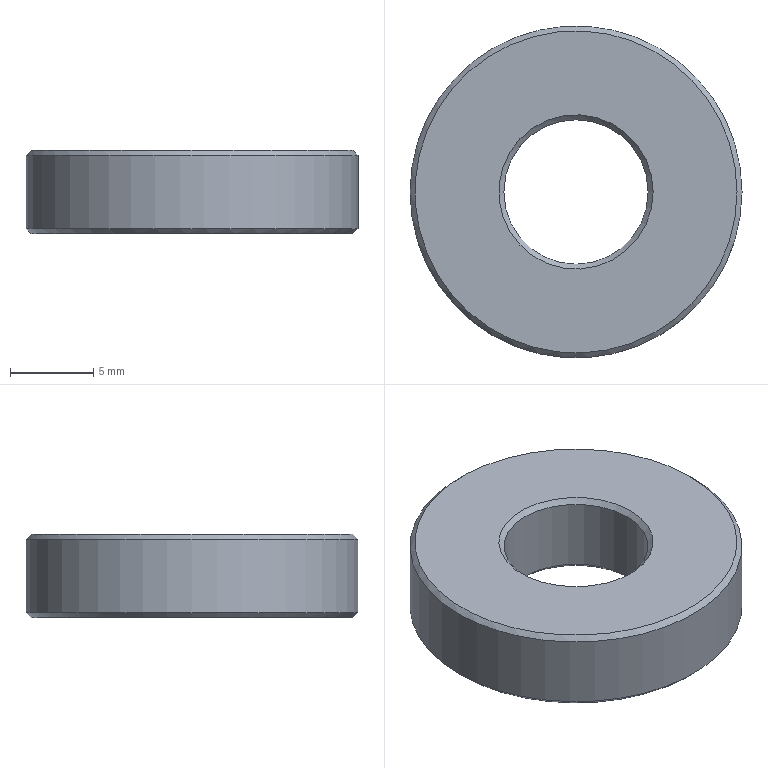Part | STEP file | 1 solid | 8 faces | box 20 x 20 x 5 mm | volume 1265 mm3 | cone 4 | plane 2 | cylinder 2 | commonest cylinder face diameters 8.7 x1 20 x1
STEP:
#1=CARTESIAN_POINT('',(0.,0.,0.));
#2=DIRECTION('',(0.,0.,1.));
#3=DIRECTION('',(1.,0.,0.));
#4=AXIS2_PLACEMENT_3D('',#1,#2,#3);
#5=CARTESIAN_POINT('',(1432.597,532.48,-85.381));
#6=VERTEX_POINT('',#5);
#7=CARTESIAN_POINT('',(1437.247,532.48,-85.381));
#8=DIRECTION('',(0.,0.,1.));
#9=DIRECTION('',(-1.,0.,0.));
#10=AXIS2_PLACEMENT_3D('',#7,#8,#9);
#11=CIRCLE('',#10,4.65);
#12=CARTESIAN_POINT('',(1437.247,532.48,-85.381));
#13=DIRECTION('',(0.,0.,-1.));
#14=DIRECTION('',(1.,0.,0.));
#15=AXIS2_PLACEMENT_3D('',#12,#13,#14);
#16=PLANE('',#15);
#17=CARTESIAN_POINT('',(-4.65,0.));
#18=CARTESIAN_POINT('',(-4.65,8.054));
#19=CARTESIAN_POINT('',(2.325,4.027));
#20=CARTESIAN_POINT('',(9.3,0.));
#21=CARTESIAN_POINT('',(2.325,-4.027));
#22=CARTESIAN_POINT('',(-4.65,-8.054));
#23=CARTESIAN_POINT('',(-4.65,0.));
#24=(BOUNDED_CURVE()B_SPLINE_CURVE(2,(#17,#18,#19,#20,#21,#22,#23),.UNSPECIFIED.,.T.,.F.)B_SPLINE_CURVE_WITH_KNOTS((1,2,2,2,2,1),(-2.094,0.,2.094,4.189,6.283,8.378),.UNSPECIFIED.)CURVE()GEOMETRIC_REPRESENTATION_ITEM()RATIONAL_B_SPLINE_CURVE((1.,0.5,1.,0.5,1.,0.5,1.))REPRESENTATION_ITEM(''));
#25=(GEOMETRIC_REPRESENTATION_CONTEXT(2)PARAMETRIC_REPRESENTATION_CONTEXT()REPRESENTATION_CONTEXT('',''));
#26=DEFINITIONAL_REPRESENTATION('',(#24),#25);
#27=PCURVE('',#16,#26);
#28=CARTESIAN_POINT('',(1437.247,532.48,-85.381));
#29=DIRECTION('',(0.,0.,-1.));
#30=DIRECTION('',(-1.,0.,0.));
#31=AXIS2_PLACEMENT_3D('',#28,#29,#30);
#32=CONICAL_SURFACE('',#31,4.65,0.7854);
#33=CARTESIAN_POINT('',(6.283,0.));
#34=DIRECTION('',(-1.,0.));
#35=VECTOR('',#34,1.);
#36=LINE('',#33,#35);
#37=(GEOMETRIC_REPRESENTATION_CONTEXT(2)PARAMETRIC_REPRESENTATION_CONTEXT()REPRESENTATION_CONTEXT('',''));
#38=DEFINITIONAL_REPRESENTATION('',(#36),#37);
#39=PCURVE('',#32,#38);
#40=SURFACE_CURVE('',#11,(#27,#39),.PCURVE_S1.);
#41=EDGE_CURVE('',#6,#6,#40,.T.);
#42=ORIENTED_EDGE('',*,*,#41,.T.);
#43=EDGE_LOOP('',(#42));
#44=FACE_BOUND('',#43,.T.);
#45=CARTESIAN_POINT('',(1427.547,532.48,-85.381));
#46=VERTEX_POINT('',#45);
#47=CARTESIAN_POINT('',(1437.247,532.48,-85.381));
#48=DIRECTION('',(0.,0.,-1.));
#49=DIRECTION('',(-1.,0.,0.));
#50=AXIS2_PLACEMENT_3D('',#47,#48,#49);
#51=CIRCLE('',#50,9.7);
#52=CARTESIAN_POINT('',(0.,0.));
#53=DIRECTION('',(-1.,0.));
#54=AXIS2_PLACEMENT_2D('',#52,#53);
#55=CIRCLE('',#54,9.7);
#56=(GEOMETRIC_REPRESENTATION_CONTEXT(2)PARAMETRIC_REPRESENTATION_CONTEXT()REPRESENTATION_CONTEXT('',''));
#57=DEFINITIONAL_REPRESENTATION('',(#55),#56);
#58=PCURVE('',#16,#57);
#59=CARTESIAN_POINT('',(1437.247,532.48,-85.081));
#60=DIRECTION('',(0.,0.,1.));
#61=DIRECTION('',(1.,0.,0.));
#62=AXIS2_PLACEMENT_3D('',#59,#60,#61);
#63=CONICAL_SURFACE('',#62,10.,0.7854);
#64=CARTESIAN_POINT('',(9.425,-0.3));
#65=DIRECTION('',(-1.,0.));
#66=VECTOR('',#65,1.);
#67=LINE('',#64,#66);
#68=(GEOMETRIC_REPRESENTATION_CONTEXT(2)PARAMETRIC_REPRESENTATION_CONTEXT()REPRESENTATION_CONTEXT('',''));
#69=DEFINITIONAL_REPRESENTATION('',(#67),#68);
#70=PCURVE('',#63,#69);
#71=SURFACE_CURVE('',#51,(#58,#70),.PCURVE_S1.);
#72=EDGE_CURVE('',#46,#46,#71,.T.);
#73=ORIENTED_EDGE('',*,*,#72,.T.);
#74=EDGE_LOOP('',(#73));
#75=FACE_BOUND('',#74,.T.);
#76=ADVANCED_FACE('',(#44,#75),#16,.T.);
#77=CARTESIAN_POINT('',(1447.247,532.48,-80.681));
#78=VERTEX_POINT('',#77);
#79=CARTESIAN_POINT('',(1427.247,532.48,-80.681));
#80=VERTEX_POINT('',#79);
#81=CARTESIAN_POINT('',(1437.247,532.48,-80.681));
#82=DIRECTION('',(0.,0.,-1.));
#83=DIRECTION('',(1.,0.,0.));
#84=AXIS2_PLACEMENT_3D('',#81,#82,#83);
#85=CIRCLE('',#84,10.);
#86=CARTESIAN_POINT('',(1437.247,532.48,-83.381));
#87=DIRECTION('',(0.,0.,-1.));
#88=DIRECTION('',(-1.,0.,0.));
#89=AXIS2_PLACEMENT_3D('',#86,#87,#88);
#90=CYLINDRICAL_SURFACE('',#89,10.);
#91=CARTESIAN_POINT('',(3.142,-2.7));
#92=DIRECTION('',(1.,0.));
#93=VECTOR('',#92,1.);
#94=LINE('',#91,#93);
#95=(GEOMETRIC_REPRESENTATION_CONTEXT(2)PARAMETRIC_REPRESENTATION_CONTEXT()REPRESENTATION_CONTEXT('',''));
#96=DEFINITIONAL_REPRESENTATION('',(#94),#95);
#97=PCURVE('',#90,#96);
#98=CARTESIAN_POINT('',(1437.247,532.48,-80.681));
#99=DIRECTION('',(0.,0.,-1.));
#100=DIRECTION('',(-1.,0.,0.));
#101=AXIS2_PLACEMENT_3D('',#98,#99,#100);
#102=CONICAL_SURFACE('',#101,10.,0.7854);
#103=CARTESIAN_POINT('',(3.142,0.));
#104=DIRECTION('',(1.,0.));
#105=VECTOR('',#104,1.);
#106=LINE('',#103,#105);
#107=(GEOMETRIC_REPRESENTATION_CONTEXT(2)PARAMETRIC_REPRESENTATION_CONTEXT()REPRESENTATION_CONTEXT('',''));
#108=DEFINITIONAL_REPRESENTATION('',(#106),#107);
#109=PCURVE('',#102,#108);
#110=SURFACE_CURVE('',#85,(#97,#109),.PCURVE_S1.);
#111=EDGE_CURVE('',#78,#80,#110,.T.);
#112=ORIENTED_EDGE('',*,*,#111,.T.);
#113=CARTESIAN_POINT('',(1427.247,532.48,-85.081));
#114=VERTEX_POINT('',#113);
#115=CARTESIAN_POINT('',(1427.247,532.48,-80.681));
#116=CARTESIAN_POINT('',(1427.247,532.48,-85.081));
#117=B_SPLINE_CURVE_WITH_KNOTS('',1,(#115,#116),.UNSPECIFIED.,.F.,.F.,(2,2),(-2.7,1.7),.PIECEWISE_BEZIER_KNOTS.);
#118=CARTESIAN_POINT('',(6.283,0.));
#119=DIRECTION('',(0.,1.));
#120=VECTOR('',#119,1.);
#121=LINE('',#118,#120);
#122=(GEOMETRIC_REPRESENTATION_CONTEXT(2)PARAMETRIC_REPRESENTATION_CONTEXT()REPRESENTATION_CONTEXT('',''));
#123=DEFINITIONAL_REPRESENTATION('',(#121),#122);
#124=PCURVE('',#90,#123);
#125=CARTESIAN_POINT('',(0.,0.));
#126=DIRECTION('',(0.,1.));
#127=VECTOR('',#126,1.);
#128=LINE('',#125,#127);
#129=(GEOMETRIC_REPRESENTATION_CONTEXT(2)PARAMETRIC_REPRESENTATION_CONTEXT()REPRESENTATION_CONTEXT('',''));
#130=DEFINITIONAL_REPRESENTATION('',(#128),#129);
#131=PCURVE('',#90,#130);
#132=SEAM_CURVE('',#117,(#124,#131),.PCURVE_S1.);
#133=EDGE_CURVE('',#80,#114,#132,.T.);
#134=ORIENTED_EDGE('',*,*,#133,.T.);
#135=CARTESIAN_POINT('',(1437.247,532.48,-85.081));
#136=DIRECTION('',(0.,0.,1.));
#137=DIRECTION('',(-1.,0.,0.));
#138=AXIS2_PLACEMENT_3D('',#135,#136,#137);
#139=CIRCLE('',#138,10.);
#140=CARTESIAN_POINT('',(6.283,1.7));
#141=DIRECTION('',(-1.,0.));
#142=VECTOR('',#141,1.);
#143=LINE('',#140,#142);
#144=(GEOMETRIC_REPRESENTATION_CONTEXT(2)PARAMETRIC_REPRESENTATION_CONTEXT()REPRESENTATION_CONTEXT('',''));
#145=DEFINITIONAL_REPRESENTATION('',(#143),#144);
#146=PCURVE('',#90,#145);
#147=CARTESIAN_POINT('',(3.142,0.));
#148=DIRECTION('',(1.,0.));
#149=VECTOR('',#148,1.);
#150=LINE('',#147,#149);
#151=(GEOMETRIC_REPRESENTATION_CONTEXT(2)PARAMETRIC_REPRESENTATION_CONTEXT()REPRESENTATION_CONTEXT('',''));
#152=DEFINITIONAL_REPRESENTATION('',(#150),#151);
#153=PCURVE('',#63,#152);
#154=SURFACE_CURVE('',#139,(#146,#153),.PCURVE_S1.);
#155=EDGE_CURVE('',#114,#114,#154,.T.);
#156=ORIENTED_EDGE('',*,*,#155,.T.);
#157=ORIENTED_EDGE('',*,*,#133,.F.);
#158=CARTESIAN_POINT('',(1437.247,532.48,-80.681));
#159=DIRECTION('',(0.,0.,-1.));
#160=DIRECTION('',(1.,0.,0.));
#161=AXIS2_PLACEMENT_3D('',#158,#159,#160);
#162=CIRCLE('',#161,10.);
#163=CARTESIAN_POINT('',(-3.142,-2.7));
#164=DIRECTION('',(1.,0.));
#165=VECTOR('',#164,1.);
#166=LINE('',#163,#165);
#167=(GEOMETRIC_REPRESENTATION_CONTEXT(2)PARAMETRIC_REPRESENTATION_CONTEXT()REPRESENTATION_CONTEXT('',''));
#168=DEFINITIONAL_REPRESENTATION('',(#166),#167);
#169=PCURVE('',#90,#168);
#170=CARTESIAN_POINT('',(3.142,0.));
#171=DIRECTION('',(1.,0.));
#172=VECTOR('',#171,1.);
#173=LINE('',#170,#172);
#174=(GEOMETRIC_REPRESENTATION_CONTEXT(2)PARAMETRIC_REPRESENTATION_CONTEXT()REPRESENTATION_CONTEXT('',''));
#175=DEFINITIONAL_REPRESENTATION('',(#173),#174);
#176=PCURVE('',#102,#175);
#177=SURFACE_CURVE('',#162,(#169,#176),.PCURVE_S1.);
#178=EDGE_CURVE('',#80,#78,#177,.T.);
#179=ORIENTED_EDGE('',*,*,#178,.T.);
#180=EDGE_LOOP('',(#112,#134,#156,#157,#179));
#181=FACE_BOUND('',#180,.T.);
#182=ADVANCED_FACE('',(#181),#90,.T.);
#183=CARTESIAN_POINT('',(1432.897,532.48,-85.081));
#184=VERTEX_POINT('',#183);
#185=CARTESIAN_POINT('',(1437.247,532.48,-85.081));
#186=DIRECTION('',(0.,0.,-1.));
#187=DIRECTION('',(-1.,0.,0.));
#188=AXIS2_PLACEMENT_3D('',#185,#186,#187);
#189=CIRCLE('',#188,4.35);
#190=CARTESIAN_POINT('',(1437.247,532.48,-89.381));
#191=DIRECTION('',(0.,0.,1.));
#192=DIRECTION('',(-1.,0.,0.));
#193=AXIS2_PLACEMENT_3D('',#190,#191,#192);
#194=CYLINDRICAL_SURFACE('',#193,4.35);
#195=CARTESIAN_POINT('',(6.283,4.3));
#196=DIRECTION('',(-1.,0.));
#197=VECTOR('',#196,1.);
#198=LINE('',#195,#197);
#199=(GEOMETRIC_REPRESENTATION_CONTEXT(2)PARAMETRIC_REPRESENTATION_CONTEXT()REPRESENTATION_CONTEXT('',''));
#200=DEFINITIONAL_REPRESENTATION('',(#198),#199);
#201=PCURVE('',#194,#200);
#202=CARTESIAN_POINT('',(0.,-0.3));
#203=DIRECTION('',(1.,0.));
#204=VECTOR('',#203,1.);
#205=LINE('',#202,#204);
#206=(GEOMETRIC_REPRESENTATION_CONTEXT(2)PARAMETRIC_REPRESENTATION_CONTEXT()REPRESENTATION_CONTEXT('',''));
#207=DEFINITIONAL_REPRESENTATION('',(#205),#206);
#208=PCURVE('',#32,#207);
#209=SURFACE_CURVE('',#189,(#201,#208),.PCURVE_S1.);
#210=EDGE_CURVE('',#184,#184,#209,.T.);
#211=ORIENTED_EDGE('',*,*,#210,.F.);
#212=CARTESIAN_POINT('',(1432.897,532.48,-80.681));
#213=VERTEX_POINT('',#212);
#214=CARTESIAN_POINT('',(1432.897,532.48,-85.081));
#215=CARTESIAN_POINT('',(1432.897,532.48,-80.681));
#216=B_SPLINE_CURVE_WITH_KNOTS('',1,(#214,#215),.UNSPECIFIED.,.F.,.F.,(2,2),(4.3,8.7),.PIECEWISE_BEZIER_KNOTS.);
#217=CARTESIAN_POINT('',(6.283,0.));
#218=DIRECTION('',(0.,1.));
#219=VECTOR('',#218,1.);
#220=LINE('',#217,#219);
#221=(GEOMETRIC_REPRESENTATION_CONTEXT(2)PARAMETRIC_REPRESENTATION_CONTEXT()REPRESENTATION_CONTEXT('',''));
#222=DEFINITIONAL_REPRESENTATION('',(#220),#221);
#223=PCURVE('',#194,#222);
#224=CARTESIAN_POINT('',(0.,0.));
#225=DIRECTION('',(0.,1.));
#226=VECTOR('',#225,1.);
#227=LINE('',#224,#226);
#228=(GEOMETRIC_REPRESENTATION_CONTEXT(2)PARAMETRIC_REPRESENTATION_CONTEXT()REPRESENTATION_CONTEXT('',''));
#229=DEFINITIONAL_REPRESENTATION('',(#227),#228);
#230=PCURVE('',#194,#229);
#231=SEAM_CURVE('',#216,(#223,#230),.PCURVE_S1.);
#232=EDGE_CURVE('',#184,#213,#231,.T.);
#233=ORIENTED_EDGE('',*,*,#232,.T.);
#234=CARTESIAN_POINT('',(1441.597,532.48,-80.681));
#235=VERTEX_POINT('',#234);
#236=CARTESIAN_POINT('',(1437.247,532.48,-80.681));
#237=DIRECTION('',(0.,0.,1.));
#238=DIRECTION('',(1.,0.,0.));
#239=AXIS2_PLACEMENT_3D('',#236,#237,#238);
#240=CIRCLE('',#239,4.35);
#241=CARTESIAN_POINT('',(3.142,8.7));
#242=DIRECTION('',(1.,0.));
#243=VECTOR('',#242,1.);
#244=LINE('',#241,#243);
#245=(GEOMETRIC_REPRESENTATION_CONTEXT(2)PARAMETRIC_REPRESENTATION_CONTEXT()REPRESENTATION_CONTEXT('',''));
#246=DEFINITIONAL_REPRESENTATION('',(#244),#245);
#247=PCURVE('',#194,#246);
#248=CARTESIAN_POINT('',(1437.247,532.48,-80.381));
#249=DIRECTION('',(0.,0.,1.));
#250=DIRECTION('',(1.,0.,0.));
#251=AXIS2_PLACEMENT_3D('',#248,#249,#250);
#252=CONICAL_SURFACE('',#251,4.65,0.7854);
#253=CARTESIAN_POINT('',(0.,-0.3));
#254=DIRECTION('',(1.,0.));
#255=VECTOR('',#254,1.);
#256=LINE('',#253,#255);
#257=(GEOMETRIC_REPRESENTATION_CONTEXT(2)PARAMETRIC_REPRESENTATION_CONTEXT()REPRESENTATION_CONTEXT('',''));
#258=DEFINITIONAL_REPRESENTATION('',(#256),#257);
#259=PCURVE('',#252,#258);
#260=SURFACE_CURVE('',#240,(#247,#259),.PCURVE_S1.);
#261=EDGE_CURVE('',#235,#213,#260,.T.);
#262=ORIENTED_EDGE('',*,*,#261,.F.);
#263=CARTESIAN_POINT('',(1437.247,532.48,-80.681));
#264=DIRECTION('',(0.,0.,1.));
#265=DIRECTION('',(1.,0.,0.));
#266=AXIS2_PLACEMENT_3D('',#263,#264,#265);
#267=CIRCLE('',#266,4.35);
#268=CARTESIAN_POINT('',(-3.142,8.7));
#269=DIRECTION('',(1.,0.));
#270=VECTOR('',#269,1.);
#271=LINE('',#268,#270);
#272=(GEOMETRIC_REPRESENTATION_CONTEXT(2)PARAMETRIC_REPRESENTATION_CONTEXT()REPRESENTATION_CONTEXT('',''));
#273=DEFINITIONAL_REPRESENTATION('',(#271),#272);
#274=PCURVE('',#194,#273);
#275=CARTESIAN_POINT('',(0.,-0.3));
#276=DIRECTION('',(1.,0.));
#277=VECTOR('',#276,1.);
#278=LINE('',#275,#277);
#279=(GEOMETRIC_REPRESENTATION_CONTEXT(2)PARAMETRIC_REPRESENTATION_CONTEXT()REPRESENTATION_CONTEXT('',''));
#280=DEFINITIONAL_REPRESENTATION('',(#278),#279);
#281=PCURVE('',#252,#280);
#282=SURFACE_CURVE('',#267,(#274,#281),.PCURVE_S1.);
#283=EDGE_CURVE('',#213,#235,#282,.T.);
#284=ORIENTED_EDGE('',*,*,#283,.F.);
#285=ORIENTED_EDGE('',*,*,#232,.F.);
#286=EDGE_LOOP('',(#211,#233,#262,#284,#285));
#287=FACE_BOUND('',#286,.F.);
#288=ADVANCED_FACE('',(#287),#194,.F.);
#289=CARTESIAN_POINT('',(1441.897,532.48,-80.381));
#290=VERTEX_POINT('',#289);
#291=CARTESIAN_POINT('',(1437.247,532.48,-80.381));
#292=DIRECTION('',(0.,0.,-1.));
#293=DIRECTION('',(1.,0.,0.));
#294=AXIS2_PLACEMENT_3D('',#291,#292,#293);
#295=CIRCLE('',#294,4.65);
#296=CARTESIAN_POINT('',(1437.247,532.48,-80.381));
#297=DIRECTION('',(0.,0.,1.));
#298=DIRECTION('',(-1.,0.,0.));
#299=AXIS2_PLACEMENT_3D('',#296,#297,#298);
#300=PLANE('',#299);
#301=CARTESIAN_POINT('',(-4.65,0.));
#302=CARTESIAN_POINT('',(-4.65,8.054));
#303=CARTESIAN_POINT('',(2.325,4.027));
#304=CARTESIAN_POINT('',(9.3,0.));
#305=CARTESIAN_POINT('',(2.325,-4.027));
#306=CARTESIAN_POINT('',(-4.65,-8.054));
#307=CARTESIAN_POINT('',(-4.65,0.));
#308=(BOUNDED_CURVE()B_SPLINE_CURVE(2,(#301,#302,#303,#304,#305,#306,#307),.UNSPECIFIED.,.T.,.F.)B_SPLINE_CURVE_WITH_KNOTS((1,2,2,2,2,1),(-2.094,0.,2.094,4.189,6.283,8.378),.UNSPECIFIED.)CURVE()GEOMETRIC_REPRESENTATION_ITEM()RATIONAL_B_SPLINE_CURVE((1.,0.5,1.,0.5,1.,0.5,1.))REPRESENTATION_ITEM(''));
#309=(GEOMETRIC_REPRESENTATION_CONTEXT(2)PARAMETRIC_REPRESENTATION_CONTEXT()REPRESENTATION_CONTEXT('',''));
#310=DEFINITIONAL_REPRESENTATION('',(#308),#309);
#311=PCURVE('',#300,#310);
#312=CARTESIAN_POINT('',(6.283,0.));
#313=DIRECTION('',(-1.,0.));
#314=VECTOR('',#313,1.);
#315=LINE('',#312,#314);
#316=(GEOMETRIC_REPRESENTATION_CONTEXT(2)PARAMETRIC_REPRESENTATION_CONTEXT()REPRESENTATION_CONTEXT('',''));
#317=DEFINITIONAL_REPRESENTATION('',(#315),#316);
#318=PCURVE('',#252,#317);
#319=SURFACE_CURVE('',#295,(#311,#318),.PCURVE_S1.);
#320=EDGE_CURVE('',#290,#290,#319,.T.);
#321=ORIENTED_EDGE('',*,*,#320,.T.);
#322=EDGE_LOOP('',(#321));
#323=FACE_BOUND('',#322,.T.);
#324=CARTESIAN_POINT('',(1446.947,532.48,-80.381));
#325=VERTEX_POINT('',#324);
#326=CARTESIAN_POINT('',(1437.247,532.48,-80.381));
#327=DIRECTION('',(0.,0.,1.));
#328=DIRECTION('',(1.,0.,0.));
#329=AXIS2_PLACEMENT_3D('',#326,#327,#328);
#330=CIRCLE('',#329,9.7);
#331=CARTESIAN_POINT('',(0.,0.));
#332=DIRECTION('',(-1.,0.));
#333=AXIS2_PLACEMENT_2D('',#331,#332);
#334=CIRCLE('',#333,9.7);
#335=(GEOMETRIC_REPRESENTATION_CONTEXT(2)PARAMETRIC_REPRESENTATION_CONTEXT()REPRESENTATION_CONTEXT('',''));
#336=DEFINITIONAL_REPRESENTATION('',(#334),#335);
#337=PCURVE('',#300,#336);
#338=CARTESIAN_POINT('',(9.425,-0.3));
#339=DIRECTION('',(-1.,0.));
#340=VECTOR('',#339,1.);
#341=LINE('',#338,#340);
#342=(GEOMETRIC_REPRESENTATION_CONTEXT(2)PARAMETRIC_REPRESENTATION_CONTEXT()REPRESENTATION_CONTEXT('',''));
#343=DEFINITIONAL_REPRESENTATION('',(#341),#342);
#344=PCURVE('',#102,#343);
#345=SURFACE_CURVE('',#330,(#337,#344),.PCURVE_S1.);
#346=EDGE_CURVE('',#325,#325,#345,.T.);
#347=ORIENTED_EDGE('',*,*,#346,.T.);
#348=EDGE_LOOP('',(#347));
#349=FACE_BOUND('',#348,.T.);
#350=ADVANCED_FACE('',(#323,#349),#300,.T.);
#351=ORIENTED_EDGE('',*,*,#210,.T.);
#352=CARTESIAN_POINT('',(1432.897,532.48,-85.081));
#353=CARTESIAN_POINT('',(1432.597,532.48,-85.381));
#354=B_SPLINE_CURVE_WITH_KNOTS('',1,(#352,#353),.UNSPECIFIED.,.F.,.F.,(2,2),(-0.4243,0.),.PIECEWISE_BEZIER_KNOTS.);
#355=CARTESIAN_POINT('',(6.283,0.));
#356=DIRECTION('',(0.,1.));
#357=VECTOR('',#356,1.);
#358=LINE('',#355,#357);
#359=(GEOMETRIC_REPRESENTATION_CONTEXT(2)PARAMETRIC_REPRESENTATION_CONTEXT()REPRESENTATION_CONTEXT('',''));
#360=DEFINITIONAL_REPRESENTATION('',(#358),#359);
#361=PCURVE('',#32,#360);
#362=CARTESIAN_POINT('',(0.,0.));
#363=DIRECTION('',(0.,1.));
#364=VECTOR('',#363,1.);
#365=LINE('',#362,#364);
#366=(GEOMETRIC_REPRESENTATION_CONTEXT(2)PARAMETRIC_REPRESENTATION_CONTEXT()REPRESENTATION_CONTEXT('',''));
#367=DEFINITIONAL_REPRESENTATION('',(#365),#366);
#368=PCURVE('',#32,#367);
#369=SEAM_CURVE('',#354,(#361,#368),.PCURVE_S1.);
#370=EDGE_CURVE('',#184,#6,#369,.T.);
#371=ORIENTED_EDGE('',*,*,#370,.T.);
#372=ORIENTED_EDGE('',*,*,#41,.T.);
#373=ORIENTED_EDGE('',*,*,#370,.F.);
#374=EDGE_LOOP('',(#351,#371,#372,#373));
#375=FACE_BOUND('',#374,.F.);
#376=ADVANCED_FACE('',(#375),#32,.F.);
#377=ORIENTED_EDGE('',*,*,#283,.T.);
#378=CARTESIAN_POINT('',(1441.597,532.48,-80.681));
#379=CARTESIAN_POINT('',(1441.897,532.48,-80.381));
#380=B_SPLINE_CURVE_WITH_KNOTS('',1,(#378,#379),.UNSPECIFIED.,.F.,.F.,(2,2),(-0.4243,0.),.PIECEWISE_BEZIER_KNOTS.);
#381=CARTESIAN_POINT('',(6.283,0.));
#382=DIRECTION('',(0.,1.));
#383=VECTOR('',#382,1.);
#384=LINE('',#381,#383);
#385=(GEOMETRIC_REPRESENTATION_CONTEXT(2)PARAMETRIC_REPRESENTATION_CONTEXT()REPRESENTATION_CONTEXT('',''));
#386=DEFINITIONAL_REPRESENTATION('',(#384),#385);
#387=PCURVE('',#252,#386);
#388=CARTESIAN_POINT('',(0.,0.));
#389=DIRECTION('',(0.,1.));
#390=VECTOR('',#389,1.);
#391=LINE('',#388,#390);
#392=(GEOMETRIC_REPRESENTATION_CONTEXT(2)PARAMETRIC_REPRESENTATION_CONTEXT()REPRESENTATION_CONTEXT('',''));
#393=DEFINITIONAL_REPRESENTATION('',(#391),#392);
#394=PCURVE('',#252,#393);
#395=SEAM_CURVE('',#380,(#387,#394),.PCURVE_S1.);
#396=EDGE_CURVE('',#235,#290,#395,.T.);
#397=ORIENTED_EDGE('',*,*,#396,.T.);
#398=ORIENTED_EDGE('',*,*,#320,.T.);
#399=ORIENTED_EDGE('',*,*,#396,.F.);
#400=ORIENTED_EDGE('',*,*,#261,.T.);
#401=EDGE_LOOP('',(#377,#397,#398,#399,#400));
#402=FACE_BOUND('',#401,.F.);
#403=ADVANCED_FACE('',(#402),#252,.F.);
#404=ORIENTED_EDGE('',*,*,#346,.F.);
#405=CARTESIAN_POINT('',(1446.947,532.48,-80.381));
#406=CARTESIAN_POINT('',(1447.247,532.48,-80.681));
#407=B_SPLINE_CURVE_WITH_KNOTS('',1,(#405,#406),.UNSPECIFIED.,.F.,.F.,(2,2),(-0.4243,0.),.PIECEWISE_BEZIER_KNOTS.);
#408=CARTESIAN_POINT('',(9.425,0.));
#409=DIRECTION('',(0.,1.));
#410=VECTOR('',#409,1.);
#411=LINE('',#408,#410);
#412=(GEOMETRIC_REPRESENTATION_CONTEXT(2)PARAMETRIC_REPRESENTATION_CONTEXT()REPRESENTATION_CONTEXT('',''));
#413=DEFINITIONAL_REPRESENTATION('',(#411),#412);
#414=PCURVE('',#102,#413);
#415=CARTESIAN_POINT('',(3.142,0.));
#416=DIRECTION('',(0.,1.));
#417=VECTOR('',#416,1.);
#418=LINE('',#415,#417);
#419=(GEOMETRIC_REPRESENTATION_CONTEXT(2)PARAMETRIC_REPRESENTATION_CONTEXT()REPRESENTATION_CONTEXT('',''));
#420=DEFINITIONAL_REPRESENTATION('',(#418),#419);
#421=PCURVE('',#102,#420);
#422=SEAM_CURVE('',#407,(#414,#421),.PCURVE_S1.);
#423=EDGE_CURVE('',#325,#78,#422,.T.);
#424=ORIENTED_EDGE('',*,*,#423,.T.);
#425=ORIENTED_EDGE('',*,*,#178,.F.);
#426=ORIENTED_EDGE('',*,*,#111,.F.);
#427=ORIENTED_EDGE('',*,*,#423,.F.);
#428=EDGE_LOOP('',(#404,#424,#425,#426,#427));
#429=FACE_BOUND('',#428,.T.);
#430=ADVANCED_FACE('',(#429),#102,.T.);
#431=ORIENTED_EDGE('',*,*,#72,.F.);
#432=CARTESIAN_POINT('',(1427.547,532.48,-85.381));
#433=CARTESIAN_POINT('',(1427.247,532.48,-85.081));
#434=B_SPLINE_CURVE_WITH_KNOTS('',1,(#432,#433),.UNSPECIFIED.,.F.,.F.,(2,2),(-0.4243,0.),.PIECEWISE_BEZIER_KNOTS.);
#435=CARTESIAN_POINT('',(9.425,0.));
#436=DIRECTION('',(0.,1.));
#437=VECTOR('',#436,1.);
#438=LINE('',#435,#437);
#439=(GEOMETRIC_REPRESENTATION_CONTEXT(2)PARAMETRIC_REPRESENTATION_CONTEXT()REPRESENTATION_CONTEXT('',''));
#440=DEFINITIONAL_REPRESENTATION('',(#438),#439);
#441=PCURVE('',#63,#440);
#442=CARTESIAN_POINT('',(3.142,0.));
#443=DIRECTION('',(0.,1.));
#444=VECTOR('',#443,1.);
#445=LINE('',#442,#444);
#446=(GEOMETRIC_REPRESENTATION_CONTEXT(2)PARAMETRIC_REPRESENTATION_CONTEXT()REPRESENTATION_CONTEXT('',''));
#447=DEFINITIONAL_REPRESENTATION('',(#445),#446);
#448=PCURVE('',#63,#447);
#449=SEAM_CURVE('',#434,(#441,#448),.PCURVE_S1.);
#450=EDGE_CURVE('',#46,#114,#449,.T.);
#451=ORIENTED_EDGE('',*,*,#450,.T.);
#452=ORIENTED_EDGE('',*,*,#155,.F.);
#453=ORIENTED_EDGE('',*,*,#450,.F.);
#454=EDGE_LOOP('',(#431,#451,#452,#453));
#455=FACE_BOUND('',#454,.T.);
#456=ADVANCED_FACE('',(#455),#63,.T.);
#457=CLOSED_SHELL('',(#76,#182,#288,#350,#376,#403,#430,#456));
#458=MANIFOLD_SOLID_BREP('',#457);
#459=(LENGTH_UNIT()NAMED_UNIT(*)SI_UNIT(.MILLI.,.METRE.));
#460=UNCERTAINTY_MEASURE_WITH_UNIT(LENGTH_MEASURE(0.00001),#459,'','');
#461=(NAMED_UNIT(*)PLANE_ANGLE_UNIT()SI_UNIT($,.RADIAN.));
#462=(NAMED_UNIT(*)SI_UNIT($,.STERADIAN.)SOLID_ANGLE_UNIT());
#463=(GEOMETRIC_REPRESENTATION_CONTEXT(3)GLOBAL_UNCERTAINTY_ASSIGNED_CONTEXT((#460))GLOBAL_UNIT_ASSIGNED_CONTEXT((#459,#461,#462))REPRESENTATION_CONTEXT('',''));
#464=ADVANCED_BREP_SHAPE_REPRESENTATION('',(#4,#458),#463);